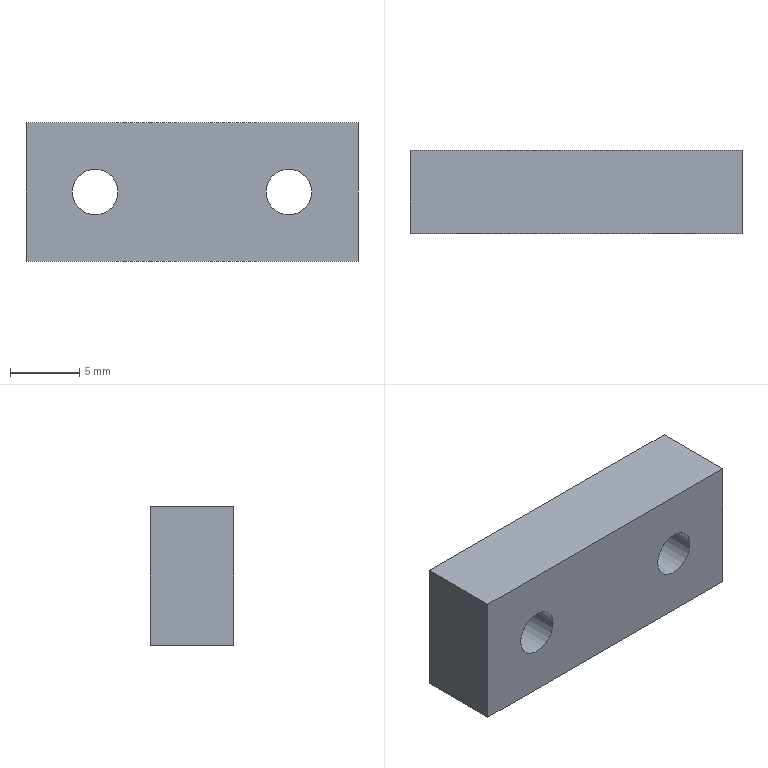Part | NX | 1 solid | 14 faces | box 24 x 6 x 10 mm | volume 1334 mm3 | plane 6 | cylinder 4 | cone 4 | commonest cylinder face diameters 3.3 x4
STEP:
#1=CARTESIAN_POINT('',(24.,0.,0.));
#2=VERTEX_POINT('',#1);
#3=CARTESIAN_POINT('',(0.,0.,0.));
#4=VERTEX_POINT('',#3);
#5=CARTESIAN_POINT('',(0.,0.,0.));
#6=DIRECTION('',(-1.,0.,0.));
#7=VECTOR('',#6,1000.);
#8=LINE('',#5,#7);
#9=EDGE_CURVE('',#2,#4,#8,.T.);
#10=ORIENTED_EDGE('',*,*,#9,.T.);
#11=CARTESIAN_POINT('',(0.,0.,-10.));
#12=VERTEX_POINT('',#11);
#13=CARTESIAN_POINT('',(0.,0.,0.));
#14=DIRECTION('',(0.,0.,-1.));
#15=VECTOR('',#14,1000.);
#16=LINE('',#13,#15);
#17=EDGE_CURVE('',#4,#12,#16,.T.);
#18=ORIENTED_EDGE('',*,*,#17,.T.);
#19=CARTESIAN_POINT('',(24.,0.,-10.));
#20=VERTEX_POINT('',#19);
#21=CARTESIAN_POINT('',(0.,0.,-10.));
#22=DIRECTION('',(1.,0.,0.));
#23=VECTOR('',#22,1000.);
#24=LINE('',#21,#23);
#25=EDGE_CURVE('',#12,#20,#24,.T.);
#26=ORIENTED_EDGE('',*,*,#25,.T.);
#27=CARTESIAN_POINT('',(24.,0.,0.));
#28=DIRECTION('',(0.,0.,1.));
#29=VECTOR('',#28,1000.);
#30=LINE('',#27,#29);
#31=EDGE_CURVE('',#20,#2,#30,.T.);
#32=ORIENTED_EDGE('',*,*,#31,.T.);
#33=EDGE_LOOP('',(#10,#18,#26,#32));
#34=FACE_BOUND('',#33,.T.);
#35=CARTESIAN_POINT('',(3.35,0.,-5.));
#36=VERTEX_POINT('',#35);
#37=CARTESIAN_POINT('',(6.65,0.,-5.));
#38=VERTEX_POINT('',#37);
#39=CARTESIAN_POINT('',(5.,0.,-5.));
#40=DIRECTION('',(0.,1.,0.));
#41=DIRECTION('',(1.,0.,0.));
#42=AXIS2_PLACEMENT_3D('',#39,#40,#41);
#43=CIRCLE('',#42,1.65);
#44=EDGE_CURVE('',#36,#38,#43,.T.);
#45=ORIENTED_EDGE('',*,*,#44,.T.);
#46=CARTESIAN_POINT('',(5.,0.,-5.));
#47=DIRECTION('',(0.,1.,0.));
#48=DIRECTION('',(1.,0.,0.));
#49=AXIS2_PLACEMENT_3D('',#46,#47,#48);
#50=CIRCLE('',#49,1.65);
#51=EDGE_CURVE('',#38,#36,#50,.T.);
#52=ORIENTED_EDGE('',*,*,#51,.T.);
#53=EDGE_LOOP('',(#45,#52));
#54=FACE_BOUND('',#53,.T.);
#55=CARTESIAN_POINT('',(17.35,0.,-5.));
#56=VERTEX_POINT('',#55);
#57=CARTESIAN_POINT('',(20.65,0.,-5.));
#58=VERTEX_POINT('',#57);
#59=CARTESIAN_POINT('',(19.,0.,-5.));
#60=DIRECTION('',(0.,1.,0.));
#61=DIRECTION('',(1.,0.,0.));
#62=AXIS2_PLACEMENT_3D('',#59,#60,#61);
#63=CIRCLE('',#62,1.65);
#64=EDGE_CURVE('',#56,#58,#63,.T.);
#65=ORIENTED_EDGE('',*,*,#64,.T.);
#66=CARTESIAN_POINT('',(19.,0.,-5.));
#67=DIRECTION('',(0.,1.,0.));
#68=DIRECTION('',(1.,0.,0.));
#69=AXIS2_PLACEMENT_3D('',#66,#67,#68);
#70=CIRCLE('',#69,1.65);
#71=EDGE_CURVE('',#58,#56,#70,.T.);
#72=ORIENTED_EDGE('',*,*,#71,.T.);
#73=EDGE_LOOP('',(#65,#72));
#74=FACE_BOUND('',#73,.T.);
#75=CARTESIAN_POINT('',(0.,0.,0.));
#76=DIRECTION('',(0.,1.,0.));
#77=DIRECTION('',(1.,0.,0.));
#78=AXIS2_PLACEMENT_3D('',#75,#76,#77);
#79=PLANE('',#78);
#80=ADVANCED_FACE('',(#34,#54,#74),#79,.F.);
#81=ORIENTED_EDGE('',*,*,#9,.F.);
#82=CARTESIAN_POINT('',(24.,6.,0.));
#83=VERTEX_POINT('',#82);
#84=CARTESIAN_POINT('',(24.,0.,0.));
#85=DIRECTION('',(0.,-1.,0.));
#86=VECTOR('',#85,1000.);
#87=LINE('',#84,#86);
#88=EDGE_CURVE('',#83,#2,#87,.T.);
#89=ORIENTED_EDGE('',*,*,#88,.F.);
#90=CARTESIAN_POINT('',(0.,6.,0.));
#91=VERTEX_POINT('',#90);
#92=CARTESIAN_POINT('',(0.,6.,0.));
#93=DIRECTION('',(1.,0.,0.));
#94=VECTOR('',#93,1000.);
#95=LINE('',#92,#94);
#96=EDGE_CURVE('',#91,#83,#95,.T.);
#97=ORIENTED_EDGE('',*,*,#96,.F.);
#98=CARTESIAN_POINT('',(0.,0.,0.));
#99=DIRECTION('',(0.,1.,0.));
#100=VECTOR('',#99,1000.);
#101=LINE('',#98,#100);
#102=EDGE_CURVE('',#4,#91,#101,.T.);
#103=ORIENTED_EDGE('',*,*,#102,.F.);
#104=EDGE_LOOP('',(#81,#89,#97,#103));
#105=FACE_BOUND('',#104,.T.);
#106=CARTESIAN_POINT('',(0.,0.,0.));
#107=DIRECTION('',(0.,0.,1.));
#108=DIRECTION('',(1.,0.,0.));
#109=AXIS2_PLACEMENT_3D('',#106,#107,#108);
#110=PLANE('',#109);
#111=ADVANCED_FACE('',(#105),#110,.T.);
#112=ORIENTED_EDGE('',*,*,#17,.F.);
#113=ORIENTED_EDGE('',*,*,#102,.T.);
#114=CARTESIAN_POINT('',(0.,6.,-10.));
#115=VERTEX_POINT('',#114);
#116=CARTESIAN_POINT('',(0.,6.,0.));
#117=DIRECTION('',(0.,0.,-1.));
#118=VECTOR('',#117,1000.);
#119=LINE('',#116,#118);
#120=EDGE_CURVE('',#91,#115,#119,.T.);
#121=ORIENTED_EDGE('',*,*,#120,.T.);
#122=CARTESIAN_POINT('',(0.,0.,-10.));
#123=DIRECTION('',(0.,-1.,0.));
#124=VECTOR('',#123,1000.);
#125=LINE('',#122,#124);
#126=EDGE_CURVE('',#115,#12,#125,.T.);
#127=ORIENTED_EDGE('',*,*,#126,.T.);
#128=EDGE_LOOP('',(#112,#113,#121,#127));
#129=FACE_BOUND('',#128,.T.);
#130=CARTESIAN_POINT('',(0.,0.,-10.));
#131=DIRECTION('',(-1.,0.,0.));
#132=DIRECTION('',(0.,0.,1.));
#133=AXIS2_PLACEMENT_3D('',#130,#131,#132);
#134=PLANE('',#133);
#135=ADVANCED_FACE('',(#129),#134,.T.);
#136=ORIENTED_EDGE('',*,*,#25,.F.);
#137=ORIENTED_EDGE('',*,*,#126,.F.);
#138=CARTESIAN_POINT('',(24.,6.,-10.));
#139=VERTEX_POINT('',#138);
#140=CARTESIAN_POINT('',(0.,6.,-10.));
#141=DIRECTION('',(1.,0.,0.));
#142=VECTOR('',#141,1000.);
#143=LINE('',#140,#142);
#144=EDGE_CURVE('',#115,#139,#143,.T.);
#145=ORIENTED_EDGE('',*,*,#144,.T.);
#146=CARTESIAN_POINT('',(24.,0.,-10.));
#147=DIRECTION('',(0.,1.,0.));
#148=VECTOR('',#147,1000.);
#149=LINE('',#146,#148);
#150=EDGE_CURVE('',#20,#139,#149,.T.);
#151=ORIENTED_EDGE('',*,*,#150,.F.);
#152=EDGE_LOOP('',(#136,#137,#145,#151));
#153=FACE_BOUND('',#152,.T.);
#154=CARTESIAN_POINT('',(10.,0.,-10.));
#155=DIRECTION('',(0.,0.,-1.));
#156=DIRECTION('',(0.,-1.,0.));
#157=AXIS2_PLACEMENT_3D('',#154,#155,#156);
#158=PLANE('',#157);
#159=ADVANCED_FACE('',(#153),#158,.T.);
#160=ORIENTED_EDGE('',*,*,#31,.F.);
#161=ORIENTED_EDGE('',*,*,#150,.T.);
#162=CARTESIAN_POINT('',(24.,6.,0.));
#163=DIRECTION('',(0.,0.,1.));
#164=VECTOR('',#163,1000.);
#165=LINE('',#162,#164);
#166=EDGE_CURVE('',#139,#83,#165,.T.);
#167=ORIENTED_EDGE('',*,*,#166,.T.);
#168=ORIENTED_EDGE('',*,*,#88,.T.);
#169=EDGE_LOOP('',(#160,#161,#167,#168));
#170=FACE_BOUND('',#169,.T.);
#171=CARTESIAN_POINT('',(24.,0.,0.));
#172=DIRECTION('',(1.,0.,0.));
#173=DIRECTION('',(0.,1.,0.));
#174=AXIS2_PLACEMENT_3D('',#171,#172,#173);
#175=PLANE('',#174);
#176=ADVANCED_FACE('',(#170),#175,.T.);
#177=ORIENTED_EDGE('',*,*,#96,.T.);
#178=ORIENTED_EDGE('',*,*,#166,.F.);
#179=ORIENTED_EDGE('',*,*,#144,.F.);
#180=ORIENTED_EDGE('',*,*,#120,.F.);
#181=EDGE_LOOP('',(#177,#178,#179,#180));
#182=FACE_BOUND('',#181,.T.);
#183=CARTESIAN_POINT('',(2.685,6.,-5.));
#184=VERTEX_POINT('',#183);
#185=CARTESIAN_POINT('',(7.315,6.,-5.));
#186=VERTEX_POINT('',#185);
#187=CARTESIAN_POINT('',(5.,6.,-5.));
#188=DIRECTION('',(0.,1.,0.));
#189=DIRECTION('',(1.,0.,0.));
#190=AXIS2_PLACEMENT_3D('',#187,#188,#189);
#191=CIRCLE('',#190,2.315);
#192=EDGE_CURVE('',#184,#186,#191,.T.);
#193=ORIENTED_EDGE('',*,*,#192,.F.);
#194=CARTESIAN_POINT('',(5.,6.,-5.));
#195=DIRECTION('',(0.,1.,0.));
#196=DIRECTION('',(1.,0.,0.));
#197=AXIS2_PLACEMENT_3D('',#194,#195,#196);
#198=CIRCLE('',#197,2.315);
#199=EDGE_CURVE('',#186,#184,#198,.T.);
#200=ORIENTED_EDGE('',*,*,#199,.F.);
#201=EDGE_LOOP('',(#193,#200));
#202=FACE_BOUND('',#201,.T.);
#203=CARTESIAN_POINT('',(21.315,6.,-5.));
#204=VERTEX_POINT('',#203);
#205=CARTESIAN_POINT('',(16.685,6.,-5.));
#206=VERTEX_POINT('',#205);
#207=CARTESIAN_POINT('',(19.,6.,-5.));
#208=DIRECTION('',(0.,1.,0.));
#209=DIRECTION('',(1.,0.,0.));
#210=AXIS2_PLACEMENT_3D('',#207,#208,#209);
#211=CIRCLE('',#210,2.315);
#212=EDGE_CURVE('',#204,#206,#211,.T.);
#213=ORIENTED_EDGE('',*,*,#212,.F.);
#214=CARTESIAN_POINT('',(19.,6.,-5.));
#215=DIRECTION('',(0.,1.,0.));
#216=DIRECTION('',(1.,0.,0.));
#217=AXIS2_PLACEMENT_3D('',#214,#215,#216);
#218=CIRCLE('',#217,2.315);
#219=EDGE_CURVE('',#206,#204,#218,.T.);
#220=ORIENTED_EDGE('',*,*,#219,.F.);
#221=EDGE_LOOP('',(#213,#220));
#222=FACE_BOUND('',#221,.T.);
#223=CARTESIAN_POINT('',(0.,6.,0.));
#224=DIRECTION('',(0.,1.,0.));
#225=DIRECTION('',(1.,0.,0.));
#226=AXIS2_PLACEMENT_3D('',#223,#224,#225);
#227=PLANE('',#226);
#228=ADVANCED_FACE('',(#182,#202,#222),#227,.T.);
#229=ORIENTED_EDGE('',*,*,#44,.F.);
#230=CARTESIAN_POINT('',(3.35,5.616,-5.));
#231=VERTEX_POINT('',#230);
#232=CARTESIAN_POINT('',(3.35,6.,-5.));
#233=DIRECTION('',(0.,1.,0.));
#234=VECTOR('',#233,1000.);
#235=LINE('',#232,#234);
#236=EDGE_CURVE('',#231,#36,#235,.F.);
#237=ORIENTED_EDGE('',*,*,#236,.F.);
#238=CARTESIAN_POINT('',(6.65,5.616,-5.));
#239=VERTEX_POINT('',#238);
#240=CARTESIAN_POINT('',(5.,5.616,-5.));
#241=DIRECTION('',(0.,1.,0.));
#242=DIRECTION('',(1.,0.,0.));
#243=AXIS2_PLACEMENT_3D('',#240,#241,#242);
#244=CIRCLE('',#243,1.65);
#245=EDGE_CURVE('',#231,#239,#244,.T.);
#246=ORIENTED_EDGE('',*,*,#245,.T.);
#247=CARTESIAN_POINT('',(6.65,6.,-5.));
#248=DIRECTION('',(0.,1.,0.));
#249=VECTOR('',#248,1000.);
#250=LINE('',#247,#249);
#251=EDGE_CURVE('',#239,#38,#250,.F.);
#252=ORIENTED_EDGE('',*,*,#251,.T.);
#253=EDGE_LOOP('',(#229,#237,#246,#252));
#254=FACE_BOUND('',#253,.T.);
#255=CARTESIAN_POINT('',(5.,6.,-5.));
#256=DIRECTION('',(0.,1.,0.));
#257=DIRECTION('',(1.,0.,0.));
#258=AXIS2_PLACEMENT_3D('',#255,#256,#257);
#259=CYLINDRICAL_SURFACE('',#258,1.65);
#260=ADVANCED_FACE('',(#254),#259,.F.);
#261=CARTESIAN_POINT('',(5.,5.616,-5.));
#262=DIRECTION('',(0.,1.,0.));
#263=DIRECTION('',(1.,0.,0.));
#264=AXIS2_PLACEMENT_3D('',#261,#262,#263);
#265=CIRCLE('',#264,1.65);
#266=EDGE_CURVE('',#239,#231,#265,.T.);
#267=ORIENTED_EDGE('',*,*,#266,.F.);
#268=CARTESIAN_POINT('',(6.65,5.616,-5.));
#269=DIRECTION('',(0.866,0.5,0.));
#270=VECTOR('',#269,1000.);
#271=LINE('',#268,#270);
#272=EDGE_CURVE('',#239,#186,#271,.T.);
#273=ORIENTED_EDGE('',*,*,#272,.T.);
#274=ORIENTED_EDGE('',*,*,#199,.T.);
#275=CARTESIAN_POINT('',(3.35,5.616,-5.));
#276=DIRECTION('',(-0.866,0.5,0.));
#277=VECTOR('',#276,1000.);
#278=LINE('',#275,#277);
#279=EDGE_CURVE('',#231,#184,#278,.T.);
#280=ORIENTED_EDGE('',*,*,#279,.F.);
#281=EDGE_LOOP('',(#267,#273,#274,#280));
#282=FACE_BOUND('',#281,.T.);
#283=CARTESIAN_POINT('',(5.,5.616,-5.));
#284=DIRECTION('',(0.,1.,0.));
#285=DIRECTION('',(1.,0.,0.));
#286=AXIS2_PLACEMENT_3D('',#283,#284,#285);
#287=CONICAL_SURFACE('',#286,1.65,1.047);
#288=ADVANCED_FACE('',(#282),#287,.F.);
#289=CARTESIAN_POINT('',(17.35,5.616,-5.));
#290=VERTEX_POINT('',#289);
#291=CARTESIAN_POINT('',(20.65,5.616,-5.));
#292=VERTEX_POINT('',#291);
#293=CARTESIAN_POINT('',(19.,5.616,-5.));
#294=DIRECTION('',(0.,1.,0.));
#295=DIRECTION('',(1.,0.,0.));
#296=AXIS2_PLACEMENT_3D('',#293,#294,#295);
#297=CIRCLE('',#296,1.65);
#298=EDGE_CURVE('',#290,#292,#297,.T.);
#299=ORIENTED_EDGE('',*,*,#298,.T.);
#300=CARTESIAN_POINT('',(20.65,6.,-5.));
#301=DIRECTION('',(0.,1.,0.));
#302=VECTOR('',#301,1000.);
#303=LINE('',#300,#302);
#304=EDGE_CURVE('',#58,#292,#303,.T.);
#305=ORIENTED_EDGE('',*,*,#304,.F.);
#306=ORIENTED_EDGE('',*,*,#64,.F.);
#307=CARTESIAN_POINT('',(17.35,6.,-5.));
#308=DIRECTION('',(0.,1.,0.));
#309=VECTOR('',#308,1000.);
#310=LINE('',#307,#309);
#311=EDGE_CURVE('',#56,#290,#310,.T.);
#312=ORIENTED_EDGE('',*,*,#311,.T.);
#313=EDGE_LOOP('',(#299,#305,#306,#312));
#314=FACE_BOUND('',#313,.T.);
#315=CARTESIAN_POINT('',(19.,6.,-5.));
#316=DIRECTION('',(0.,1.,0.));
#317=DIRECTION('',(1.,0.,0.));
#318=AXIS2_PLACEMENT_3D('',#315,#316,#317);
#319=CYLINDRICAL_SURFACE('',#318,1.65);
#320=ADVANCED_FACE('',(#314),#319,.F.);
#321=ORIENTED_EDGE('',*,*,#298,.F.);
#322=CARTESIAN_POINT('',(17.35,5.616,-5.));
#323=DIRECTION('',(-0.866,0.5,0.));
#324=VECTOR('',#323,1000.);
#325=LINE('',#322,#324);
#326=EDGE_CURVE('',#206,#290,#325,.F.);
#327=ORIENTED_EDGE('',*,*,#326,.F.);
#328=ORIENTED_EDGE('',*,*,#219,.T.);
#329=CARTESIAN_POINT('',(20.65,5.616,-5.));
#330=DIRECTION('',(0.866,0.5,0.));
#331=VECTOR('',#330,1000.);
#332=LINE('',#329,#331);
#333=EDGE_CURVE('',#204,#292,#332,.F.);
#334=ORIENTED_EDGE('',*,*,#333,.T.);
#335=EDGE_LOOP('',(#321,#327,#328,#334));
#336=FACE_BOUND('',#335,.T.);
#337=CARTESIAN_POINT('',(19.,5.616,-5.));
#338=DIRECTION('',(0.,1.,0.));
#339=DIRECTION('',(1.,0.,0.));
#340=AXIS2_PLACEMENT_3D('',#337,#338,#339);
#341=CONICAL_SURFACE('',#340,1.65,1.047);
#342=ADVANCED_FACE('',(#336),#341,.F.);
#343=ORIENTED_EDGE('',*,*,#304,.T.);
#344=CARTESIAN_POINT('',(19.,5.616,-5.));
#345=DIRECTION('',(0.,1.,0.));
#346=DIRECTION('',(1.,0.,0.));
#347=AXIS2_PLACEMENT_3D('',#344,#345,#346);
#348=CIRCLE('',#347,1.65);
#349=EDGE_CURVE('',#292,#290,#348,.T.);
#350=ORIENTED_EDGE('',*,*,#349,.T.);
#351=ORIENTED_EDGE('',*,*,#311,.F.);
#352=ORIENTED_EDGE('',*,*,#71,.F.);
#353=EDGE_LOOP('',(#343,#350,#351,#352));
#354=FACE_BOUND('',#353,.T.);
#355=CARTESIAN_POINT('',(19.,6.,-5.));
#356=DIRECTION('',(0.,1.,0.));
#357=DIRECTION('',(1.,0.,0.));
#358=AXIS2_PLACEMENT_3D('',#355,#356,#357);
#359=CYLINDRICAL_SURFACE('',#358,1.65);
#360=ADVANCED_FACE('',(#354),#359,.F.);
#361=ORIENTED_EDGE('',*,*,#212,.T.);
#362=ORIENTED_EDGE('',*,*,#326,.T.);
#363=ORIENTED_EDGE('',*,*,#349,.F.);
#364=ORIENTED_EDGE('',*,*,#333,.F.);
#365=EDGE_LOOP('',(#361,#362,#363,#364));
#366=FACE_BOUND('',#365,.T.);
#367=CARTESIAN_POINT('',(19.,5.616,-5.));
#368=DIRECTION('',(0.,1.,0.));
#369=DIRECTION('',(1.,0.,0.));
#370=AXIS2_PLACEMENT_3D('',#367,#368,#369);
#371=CONICAL_SURFACE('',#370,1.65,1.047);
#372=ADVANCED_FACE('',(#366),#371,.F.);
#373=ORIENTED_EDGE('',*,*,#266,.T.);
#374=ORIENTED_EDGE('',*,*,#236,.T.);
#375=ORIENTED_EDGE('',*,*,#51,.F.);
#376=ORIENTED_EDGE('',*,*,#251,.F.);
#377=EDGE_LOOP('',(#373,#374,#375,#376));
#378=FACE_BOUND('',#377,.T.);
#379=CARTESIAN_POINT('',(5.,6.,-5.));
#380=DIRECTION('',(0.,1.,0.));
#381=DIRECTION('',(1.,0.,0.));
#382=AXIS2_PLACEMENT_3D('',#379,#380,#381);
#383=CYLINDRICAL_SURFACE('',#382,1.65);
#384=ADVANCED_FACE('',(#378),#383,.F.);
#385=ORIENTED_EDGE('',*,*,#192,.T.);
#386=ORIENTED_EDGE('',*,*,#272,.F.);
#387=ORIENTED_EDGE('',*,*,#245,.F.);
#388=ORIENTED_EDGE('',*,*,#279,.T.);
#389=EDGE_LOOP('',(#385,#386,#387,#388));
#390=FACE_BOUND('',#389,.T.);
#391=CARTESIAN_POINT('',(5.,5.616,-5.));
#392=DIRECTION('',(0.,1.,0.));
#393=DIRECTION('',(1.,0.,0.));
#394=AXIS2_PLACEMENT_3D('',#391,#392,#393);
#395=CONICAL_SURFACE('',#394,1.65,1.047);
#396=ADVANCED_FACE('',(#390),#395,.F.);
#397=CLOSED_SHELL('',(#80,#111,#135,#159,#176,#228,#260,#288,#320,#342,#360,#372,#384,#396));
#398=MANIFOLD_SOLID_BREP('',#397);
#399=(LENGTH_UNIT()NAMED_UNIT(*)SI_UNIT(.MILLI.,.METRE.));
#400=UNCERTAINTY_MEASURE_WITH_UNIT(LENGTH_MEASURE(0.00001),#399,'','');
#401=(NAMED_UNIT(*)PLANE_ANGLE_UNIT()SI_UNIT($,.RADIAN.));
#402=(NAMED_UNIT(*)SI_UNIT($,.STERADIAN.)SOLID_ANGLE_UNIT());
#403=(GEOMETRIC_REPRESENTATION_CONTEXT(3)GLOBAL_UNCERTAINTY_ASSIGNED_CONTEXT((#400))GLOBAL_UNIT_ASSIGNED_CONTEXT((#399,#401,#402))REPRESENTATION_CONTEXT('',''));
#404=ADVANCED_BREP_SHAPE_REPRESENTATION('',(#398),#403);